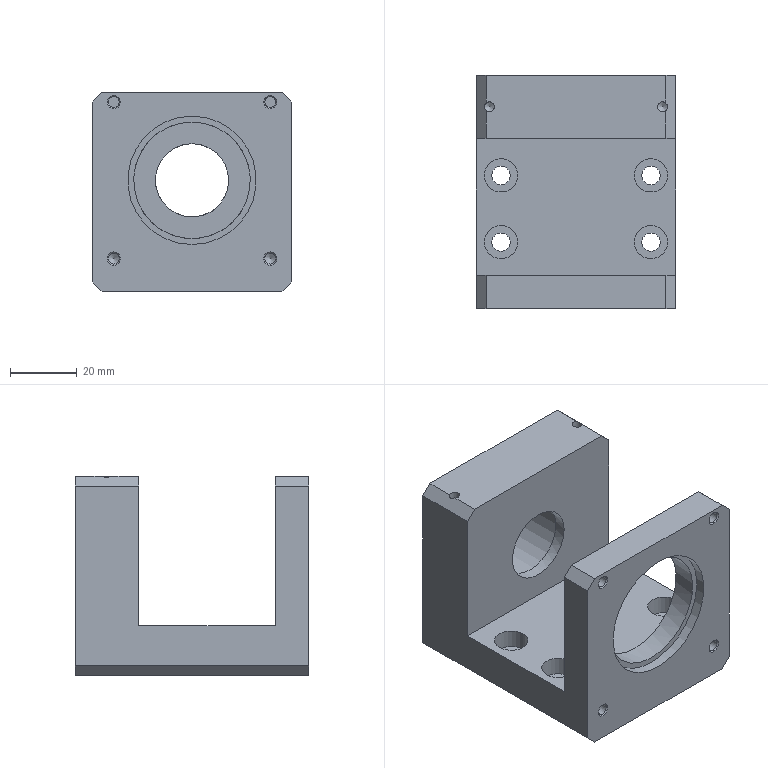Part | NX | 1 solid | 62 faces | box 60 x 70 x 60 mm | volume 117109 mm3 | cylinder 22 | plane 22 | cone 18 | commonest cylinder face diameters 3 x6 3.3 x4 5.5 x4 10 x4 22 x1 26 x1
STEP:
#1=CARTESIAN_POINT('',(41.,-19.,33.5));
#2=VERTEX_POINT('',#1);
#3=CARTESIAN_POINT('',(30.,-19.,33.5));
#4=DIRECTION('',(0.,1.,0.));
#5=DIRECTION('',(1.,0.,0.));
#6=AXIS2_PLACEMENT_3D('',#3,#4,#5);
#7=CIRCLE('',#6,11.);
#8=EDGE_CURVE('',#2,#2,#7,.T.);
#9=ORIENTED_EDGE('',*,*,#8,.F.);
#10=EDGE_LOOP('',(#9));
#11=FACE_BOUND('',#10,.T.);
#12=CARTESIAN_POINT('',(30.,-15.5,44.5));
#13=VERTEX_POINT('',#12);
#14=CARTESIAN_POINT('',(30.,-15.5,33.5));
#15=DIRECTION('',(0.,1.,0.));
#16=DIRECTION('',(0.,0.,1.));
#17=AXIS2_PLACEMENT_3D('',#14,#15,#16);
#18=CIRCLE('',#17,11.);
#19=EDGE_CURVE('',#13,#13,#18,.T.);
#20=ORIENTED_EDGE('',*,*,#19,.T.);
#21=EDGE_LOOP('',(#20));
#22=FACE_BOUND('',#21,.T.);
#23=CARTESIAN_POINT('',(30.,30.,33.5));
#24=DIRECTION('',(0.,-1.,0.));
#25=DIRECTION('',(0.,0.,1.));
#26=AXIS2_PLACEMENT_3D('',#23,#24,#25);
#27=CYLINDRICAL_SURFACE('',#26,11.);
#28=ADVANCED_FACE('',(#11,#22),#27,.F.);
#29=CARTESIAN_POINT('',(55.25,-30.,0.));
#30=VERTEX_POINT('',#29);
#31=CARTESIAN_POINT('',(52.5,-30.,0.));
#32=DIRECTION('',(0.,0.,1.));
#33=DIRECTION('',(1.,0.,0.));
#34=AXIS2_PLACEMENT_3D('',#31,#32,#33);
#35=CIRCLE('',#34,2.75);
#36=EDGE_CURVE('',#30,#30,#35,.T.);
#37=ORIENTED_EDGE('',*,*,#36,.F.);
#38=EDGE_LOOP('',(#37));
#39=FACE_BOUND('',#38,.T.);
#40=CARTESIAN_POINT('',(55.25,-30.,9.3));
#41=VERTEX_POINT('',#40);
#42=CARTESIAN_POINT('',(52.5,-30.,9.3));
#43=DIRECTION('',(0.,0.,-1.));
#44=DIRECTION('',(1.,0.,0.));
#45=AXIS2_PLACEMENT_3D('',#42,#43,#44);
#46=CIRCLE('',#45,2.75);
#47=EDGE_CURVE('',#41,#41,#46,.T.);
#48=ORIENTED_EDGE('',*,*,#47,.F.);
#49=EDGE_LOOP('',(#48));
#50=FACE_BOUND('',#49,.T.);
#51=CARTESIAN_POINT('',(52.5,-30.,-140.));
#52=DIRECTION('',(0.,0.,1.));
#53=DIRECTION('',(-1.,0.,0.));
#54=AXIS2_PLACEMENT_3D('',#51,#52,#53);
#55=CYLINDRICAL_SURFACE('',#54,2.75);
#56=ADVANCED_FACE('',(#39,#50),#55,.F.);
#57=CARTESIAN_POINT('',(10.25,-50.,0.));
#58=VERTEX_POINT('',#57);
#59=CARTESIAN_POINT('',(7.5,-50.,0.));
#60=DIRECTION('',(0.,0.,1.));
#61=DIRECTION('',(1.,0.,0.));
#62=AXIS2_PLACEMENT_3D('',#59,#60,#61);
#63=CIRCLE('',#62,2.75);
#64=EDGE_CURVE('',#58,#58,#63,.T.);
#65=ORIENTED_EDGE('',*,*,#64,.F.);
#66=EDGE_LOOP('',(#65));
#67=FACE_BOUND('',#66,.T.);
#68=CARTESIAN_POINT('',(10.25,-50.,9.3));
#69=VERTEX_POINT('',#68);
#70=CARTESIAN_POINT('',(7.5,-50.,9.3));
#71=DIRECTION('',(0.,0.,-1.));
#72=DIRECTION('',(1.,0.,0.));
#73=AXIS2_PLACEMENT_3D('',#70,#71,#72);
#74=CIRCLE('',#73,2.75);
#75=EDGE_CURVE('',#69,#69,#74,.T.);
#76=ORIENTED_EDGE('',*,*,#75,.F.);
#77=EDGE_LOOP('',(#76));
#78=FACE_BOUND('',#77,.T.);
#79=CARTESIAN_POINT('',(7.5,-50.,-140.));
#80=DIRECTION('',(0.,0.,1.));
#81=DIRECTION('',(-1.,0.,0.));
#82=AXIS2_PLACEMENT_3D('',#79,#80,#81);
#83=CYLINDRICAL_SURFACE('',#82,2.75);
#84=ADVANCED_FACE('',(#67,#78),#83,.F.);
#85=CARTESIAN_POINT('',(10.25,-30.,0.));
#86=VERTEX_POINT('',#85);
#87=CARTESIAN_POINT('',(7.5,-30.,0.));
#88=DIRECTION('',(0.,0.,1.));
#89=DIRECTION('',(1.,0.,0.));
#90=AXIS2_PLACEMENT_3D('',#87,#88,#89);
#91=CIRCLE('',#90,2.75);
#92=EDGE_CURVE('',#86,#86,#91,.T.);
#93=ORIENTED_EDGE('',*,*,#92,.F.);
#94=EDGE_LOOP('',(#93));
#95=FACE_BOUND('',#94,.T.);
#96=CARTESIAN_POINT('',(10.25,-30.,9.3));
#97=VERTEX_POINT('',#96);
#98=CARTESIAN_POINT('',(7.5,-30.,9.3));
#99=DIRECTION('',(0.,0.,-1.));
#100=DIRECTION('',(1.,0.,0.));
#101=AXIS2_PLACEMENT_3D('',#98,#99,#100);
#102=CIRCLE('',#101,2.75);
#103=EDGE_CURVE('',#97,#97,#102,.T.);
#104=ORIENTED_EDGE('',*,*,#103,.F.);
#105=EDGE_LOOP('',(#104));
#106=FACE_BOUND('',#105,.T.);
#107=CARTESIAN_POINT('',(7.5,-30.,-140.));
#108=DIRECTION('',(0.,0.,1.));
#109=DIRECTION('',(-1.,0.,0.));
#110=AXIS2_PLACEMENT_3D('',#107,#108,#109);
#111=CYLINDRICAL_SURFACE('',#110,2.75);
#112=ADVANCED_FACE('',(#95,#106),#111,.F.);
#113=CARTESIAN_POINT('',(55.25,-50.,0.));
#114=VERTEX_POINT('',#113);
#115=CARTESIAN_POINT('',(52.5,-50.,0.));
#116=DIRECTION('',(0.,0.,1.));
#117=DIRECTION('',(1.,0.,0.));
#118=AXIS2_PLACEMENT_3D('',#115,#116,#117);
#119=CIRCLE('',#118,2.75);
#120=EDGE_CURVE('',#114,#114,#119,.T.);
#121=ORIENTED_EDGE('',*,*,#120,.F.);
#122=EDGE_LOOP('',(#121));
#123=FACE_BOUND('',#122,.T.);
#124=CARTESIAN_POINT('',(55.25,-50.,9.3));
#125=VERTEX_POINT('',#124);
#126=CARTESIAN_POINT('',(52.5,-50.,9.3));
#127=DIRECTION('',(0.,0.,-1.));
#128=DIRECTION('',(1.,0.,0.));
#129=AXIS2_PLACEMENT_3D('',#126,#127,#128);
#130=CIRCLE('',#129,2.75);
#131=EDGE_CURVE('',#125,#125,#130,.T.);
#132=ORIENTED_EDGE('',*,*,#131,.F.);
#133=EDGE_LOOP('',(#132));
#134=FACE_BOUND('',#133,.T.);
#135=CARTESIAN_POINT('',(52.5,-50.,-140.));
#136=DIRECTION('',(0.,0.,1.));
#137=DIRECTION('',(-1.,0.,0.));
#138=AXIS2_PLACEMENT_3D('',#135,#136,#137);
#139=CYLINDRICAL_SURFACE('',#138,2.75);
#140=ADVANCED_FACE('',(#123,#134),#139,.F.);
#141=CARTESIAN_POINT('',(57.,-60.,60.));
#142=VERTEX_POINT('',#141);
#143=CARTESIAN_POINT('',(57.,-70.,60.));
#144=VERTEX_POINT('',#143);
#145=CARTESIAN_POINT('',(57.,0.,60.));
#146=DIRECTION('',(0.,-1.,0.));
#147=VECTOR('',#146,1.);
#148=LINE('',#145,#147);
#149=EDGE_CURVE('',#142,#144,#148,.T.);
#150=ORIENTED_EDGE('',*,*,#149,.F.);
#151=CARTESIAN_POINT('',(3.,-60.,60.));
#152=VERTEX_POINT('',#151);
#153=CARTESIAN_POINT('',(60.,-60.,60.));
#154=DIRECTION('',(-1.,0.,0.));
#155=VECTOR('',#154,1.);
#156=LINE('',#153,#155);
#157=EDGE_CURVE('',#142,#152,#156,.T.);
#158=ORIENTED_EDGE('',*,*,#157,.T.);
#159=CARTESIAN_POINT('',(3.,-70.,60.));
#160=VERTEX_POINT('',#159);
#161=CARTESIAN_POINT('',(3.,0.,60.));
#162=DIRECTION('',(0.,-1.,0.));
#163=VECTOR('',#162,1.);
#164=LINE('',#161,#163);
#165=EDGE_CURVE('',#152,#160,#164,.T.);
#166=ORIENTED_EDGE('',*,*,#165,.T.);
#167=CARTESIAN_POINT('',(3.,-70.,60.));
#168=DIRECTION('',(1.,0.,0.));
#169=VECTOR('',#168,1.);
#170=LINE('',#167,#169);
#171=EDGE_CURVE('',#160,#144,#170,.T.);
#172=ORIENTED_EDGE('',*,*,#171,.T.);
#173=EDGE_LOOP('',(#150,#158,#166,#172));
#174=FACE_OUTER_BOUND('',#173,.T.);
#175=CARTESIAN_POINT('',(3.,0.,60.));
#176=DIRECTION('',(0.,0.,-1.));
#177=DIRECTION('',(1.,0.,0.));
#178=AXIS2_PLACEMENT_3D('',#175,#176,#177);
#179=PLANE('',#178);
#180=ADVANCED_FACE('',(#174),#179,.F.);
#181=CARTESIAN_POINT('',(57.,0.,60.));
#182=VERTEX_POINT('',#181);
#183=CARTESIAN_POINT('',(57.,-8.382,60.));
#184=VERTEX_POINT('',#183);
#185=CARTESIAN_POINT('',(57.,0.,60.));
#186=DIRECTION('',(0.,-1.,0.));
#187=VECTOR('',#186,1.);
#188=LINE('',#185,#187);
#189=EDGE_CURVE('',#182,#184,#188,.T.);
#190=ORIENTED_EDGE('',*,*,#189,.T.);
#191=CARTESIAN_POINT('',(57.,-10.618,60.));
#192=VERTEX_POINT('',#191);
#193=CARTESIAN_POINT('',(56.,-9.5,61.));
#194=DIRECTION('',(-0.7071,0.,-0.7071));
#195=DIRECTION('',(0.7071,0.,-0.7071));
#196=AXIS2_PLACEMENT_3D('',#193,#194,#195);
#197=ELLIPSE('',#196,2.121,1.5);
#198=EDGE_CURVE('',#184,#192,#197,.T.);
#199=ORIENTED_EDGE('',*,*,#198,.T.);
#200=CARTESIAN_POINT('',(57.,-19.,60.));
#201=VERTEX_POINT('',#200);
#202=CARTESIAN_POINT('',(57.,0.,60.));
#203=DIRECTION('',(0.,-1.,0.));
#204=VECTOR('',#203,1.);
#205=LINE('',#202,#204);
#206=EDGE_CURVE('',#192,#201,#205,.T.);
#207=ORIENTED_EDGE('',*,*,#206,.T.);
#208=CARTESIAN_POINT('',(60.,-19.,57.));
#209=VERTEX_POINT('',#208);
#210=CARTESIAN_POINT('',(57.,-19.,60.));
#211=DIRECTION('',(-0.7071,0.,0.7071));
#212=VECTOR('',#211,1.);
#213=LINE('',#210,#212);
#214=EDGE_CURVE('',#209,#201,#213,.T.);
#215=ORIENTED_EDGE('',*,*,#214,.F.);
#216=CARTESIAN_POINT('',(60.,0.,57.));
#217=VERTEX_POINT('',#216);
#218=CARTESIAN_POINT('',(60.,0.,57.));
#219=DIRECTION('',(0.,-1.,0.));
#220=VECTOR('',#219,1.);
#221=LINE('',#218,#220);
#222=EDGE_CURVE('',#217,#209,#221,.T.);
#223=ORIENTED_EDGE('',*,*,#222,.F.);
#224=CARTESIAN_POINT('',(57.,0.,60.));
#225=DIRECTION('',(0.7071,0.,-0.7071));
#226=VECTOR('',#225,1.);
#227=LINE('',#224,#226);
#228=EDGE_CURVE('',#182,#217,#227,.T.);
#229=ORIENTED_EDGE('',*,*,#228,.F.);
#230=EDGE_LOOP('',(#190,#199,#207,#215,#223,#229));
#231=FACE_OUTER_BOUND('',#230,.T.);
#232=CARTESIAN_POINT('',(57.,0.,60.));
#233=DIRECTION('',(-0.7071,0.,-0.7071));
#234=DIRECTION('',(0.7071,0.,-0.7071));
#235=AXIS2_PLACEMENT_3D('',#232,#233,#234);
#236=PLANE('',#235);
#237=ADVANCED_FACE('',(#231),#236,.F.);
#238=CARTESIAN_POINT('',(60.,-60.,57.));
#239=VERTEX_POINT('',#238);
#240=CARTESIAN_POINT('',(57.,-60.,60.));
#241=DIRECTION('',(0.7071,0.,-0.7071));
#242=VECTOR('',#241,1.);
#243=LINE('',#240,#242);
#244=EDGE_CURVE('',#142,#239,#243,.T.);
#245=ORIENTED_EDGE('',*,*,#244,.F.);
#246=ORIENTED_EDGE('',*,*,#149,.T.);
#247=CARTESIAN_POINT('',(60.,-70.,57.));
#248=VERTEX_POINT('',#247);
#249=CARTESIAN_POINT('',(57.,-70.,60.));
#250=DIRECTION('',(0.7071,0.,-0.7071));
#251=VECTOR('',#250,1.);
#252=LINE('',#249,#251);
#253=EDGE_CURVE('',#144,#248,#252,.T.);
#254=ORIENTED_EDGE('',*,*,#253,.T.);
#255=CARTESIAN_POINT('',(60.,0.,57.));
#256=DIRECTION('',(0.,-1.,0.));
#257=VECTOR('',#256,1.);
#258=LINE('',#255,#257);
#259=EDGE_CURVE('',#239,#248,#258,.T.);
#260=ORIENTED_EDGE('',*,*,#259,.F.);
#261=EDGE_LOOP('',(#245,#246,#254,#260));
#262=FACE_OUTER_BOUND('',#261,.T.);
#263=CARTESIAN_POINT('',(57.,0.,60.));
#264=DIRECTION('',(-0.7071,0.,-0.7071));
#265=DIRECTION('',(0.7071,0.,-0.7071));
#266=AXIS2_PLACEMENT_3D('',#263,#264,#265);
#267=PLANE('',#266);
#268=ADVANCED_FACE('',(#262),#267,.F.);
#269=CARTESIAN_POINT('',(3.,-10.618,60.));
#270=VERTEX_POINT('',#269);
#271=CARTESIAN_POINT('',(3.,-19.,60.));
#272=VERTEX_POINT('',#271);
#273=CARTESIAN_POINT('',(3.,0.,60.));
#274=DIRECTION('',(0.,-1.,0.));
#275=VECTOR('',#274,1.);
#276=LINE('',#273,#275);
#277=EDGE_CURVE('',#270,#272,#276,.T.);
#278=ORIENTED_EDGE('',*,*,#277,.F.);
#279=CARTESIAN_POINT('',(3.,-8.382,60.));
#280=VERTEX_POINT('',#279);
#281=CARTESIAN_POINT('',(4.,-9.5,61.));
#282=DIRECTION('',(0.7071,0.,-0.7071));
#283=DIRECTION('',(-0.7071,0.,-0.7071));
#284=AXIS2_PLACEMENT_3D('',#281,#282,#283);
#285=ELLIPSE('',#284,2.121,1.5);
#286=EDGE_CURVE('',#270,#280,#285,.T.);
#287=ORIENTED_EDGE('',*,*,#286,.T.);
#288=CARTESIAN_POINT('',(3.,0.,60.));
#289=VERTEX_POINT('',#288);
#290=CARTESIAN_POINT('',(3.,0.,60.));
#291=DIRECTION('',(0.,-1.,0.));
#292=VECTOR('',#291,1.);
#293=LINE('',#290,#292);
#294=EDGE_CURVE('',#289,#280,#293,.T.);
#295=ORIENTED_EDGE('',*,*,#294,.F.);
#296=CARTESIAN_POINT('',(0.,0.,57.));
#297=VERTEX_POINT('',#296);
#298=CARTESIAN_POINT('',(0.,0.,57.));
#299=DIRECTION('',(0.7071,0.,0.7071));
#300=VECTOR('',#299,1.);
#301=LINE('',#298,#300);
#302=EDGE_CURVE('',#297,#289,#301,.T.);
#303=ORIENTED_EDGE('',*,*,#302,.F.);
#304=CARTESIAN_POINT('',(0.,-19.,57.));
#305=VERTEX_POINT('',#304);
#306=CARTESIAN_POINT('',(0.,0.,57.));
#307=DIRECTION('',(0.,-1.,0.));
#308=VECTOR('',#307,1.);
#309=LINE('',#306,#308);
#310=EDGE_CURVE('',#297,#305,#309,.T.);
#311=ORIENTED_EDGE('',*,*,#310,.T.);
#312=CARTESIAN_POINT('',(0.,-19.,57.));
#313=DIRECTION('',(-0.7071,0.,-0.7071));
#314=VECTOR('',#313,1.);
#315=LINE('',#312,#314);
#316=EDGE_CURVE('',#272,#305,#315,.T.);
#317=ORIENTED_EDGE('',*,*,#316,.F.);
#318=EDGE_LOOP('',(#278,#287,#295,#303,#311,#317));
#319=FACE_OUTER_BOUND('',#318,.T.);
#320=CARTESIAN_POINT('',(0.,0.,57.));
#321=DIRECTION('',(0.7071,0.,-0.7071));
#322=DIRECTION('',(0.7071,0.,0.7071));
#323=AXIS2_PLACEMENT_3D('',#320,#321,#322);
#324=PLANE('',#323);
#325=ADVANCED_FACE('',(#319),#324,.F.);
#326=CARTESIAN_POINT('',(0.,-60.,57.));
#327=VERTEX_POINT('',#326);
#328=CARTESIAN_POINT('',(0.,-60.,57.));
#329=DIRECTION('',(0.7071,0.,0.7071));
#330=VECTOR('',#329,1.);
#331=LINE('',#328,#330);
#332=EDGE_CURVE('',#327,#152,#331,.T.);
#333=ORIENTED_EDGE('',*,*,#332,.F.);
#334=CARTESIAN_POINT('',(0.,-70.,57.));
#335=VERTEX_POINT('',#334);
#336=CARTESIAN_POINT('',(0.,0.,57.));
#337=DIRECTION('',(0.,-1.,0.));
#338=VECTOR('',#337,1.);
#339=LINE('',#336,#338);
#340=EDGE_CURVE('',#327,#335,#339,.T.);
#341=ORIENTED_EDGE('',*,*,#340,.T.);
#342=CARTESIAN_POINT('',(0.,-70.,57.));
#343=DIRECTION('',(0.7071,0.,0.7071));
#344=VECTOR('',#343,1.);
#345=LINE('',#342,#344);
#346=EDGE_CURVE('',#335,#160,#345,.T.);
#347=ORIENTED_EDGE('',*,*,#346,.T.);
#348=ORIENTED_EDGE('',*,*,#165,.F.);
#349=EDGE_LOOP('',(#333,#341,#347,#348));
#350=FACE_OUTER_BOUND('',#349,.T.);
#351=CARTESIAN_POINT('',(0.,0.,57.));
#352=DIRECTION('',(0.7071,0.,-0.7071));
#353=DIRECTION('',(0.7071,0.,0.7071));
#354=AXIS2_PLACEMENT_3D('',#351,#352,#353);
#355=PLANE('',#354);
#356=ADVANCED_FACE('',(#350),#355,.F.);
#357=ORIENTED_EDGE('',*,*,#206,.F.);
#358=CARTESIAN_POINT('',(56.,-9.5,60.));
#359=DIRECTION('',(0.,0.,-1.));
#360=DIRECTION('',(-1.,0.,0.));
#361=AXIS2_PLACEMENT_3D('',#358,#359,#360);
#362=CIRCLE('',#361,1.5);
#363=EDGE_CURVE('',#192,#184,#362,.T.);
#364=ORIENTED_EDGE('',*,*,#363,.T.);
#365=ORIENTED_EDGE('',*,*,#189,.F.);
#366=CARTESIAN_POINT('',(3.,0.,60.));
#367=DIRECTION('',(1.,0.,0.));
#368=VECTOR('',#367,1.);
#369=LINE('',#366,#368);
#370=EDGE_CURVE('',#289,#182,#369,.T.);
#371=ORIENTED_EDGE('',*,*,#370,.F.);
#372=ORIENTED_EDGE('',*,*,#294,.T.);
#373=CARTESIAN_POINT('',(4.,-9.5,60.));
#374=DIRECTION('',(0.,0.,-1.));
#375=DIRECTION('',(-1.,0.,0.));
#376=AXIS2_PLACEMENT_3D('',#373,#374,#375);
#377=CIRCLE('',#376,1.5);
#378=EDGE_CURVE('',#280,#270,#377,.T.);
#379=ORIENTED_EDGE('',*,*,#378,.T.);
#380=ORIENTED_EDGE('',*,*,#277,.T.);
#381=CARTESIAN_POINT('',(0.,-19.,60.));
#382=DIRECTION('',(1.,0.,0.));
#383=VECTOR('',#382,1.);
#384=LINE('',#381,#383);
#385=EDGE_CURVE('',#272,#201,#384,.T.);
#386=ORIENTED_EDGE('',*,*,#385,.T.);
#387=EDGE_LOOP('',(#357,#364,#365,#371,#372,#379,#380,#386));
#388=FACE_OUTER_BOUND('',#387,.T.);
#389=CARTESIAN_POINT('',(3.,0.,60.));
#390=DIRECTION('',(0.,0.,-1.));
#391=DIRECTION('',(1.,0.,0.));
#392=AXIS2_PLACEMENT_3D('',#389,#390,#391);
#393=PLANE('',#392);
#394=ADVANCED_FACE('',(#388),#393,.F.);
#395=CARTESIAN_POINT('',(60.,-19.,15.));
#396=VERTEX_POINT('',#395);
#397=CARTESIAN_POINT('',(60.,-60.,15.));
#398=VERTEX_POINT('',#397);
#399=CARTESIAN_POINT('',(60.,-19.,15.));
#400=DIRECTION('',(0.,-1.,0.));
#401=VECTOR('',#400,1.);
#402=LINE('',#399,#401);
#403=EDGE_CURVE('',#396,#398,#402,.T.);
#404=ORIENTED_EDGE('',*,*,#403,.T.);
#405=CARTESIAN_POINT('',(60.,-60.,15.));
#406=DIRECTION('',(0.,0.,1.));
#407=VECTOR('',#406,1.);
#408=LINE('',#405,#407);
#409=EDGE_CURVE('',#398,#239,#408,.T.);
#410=ORIENTED_EDGE('',*,*,#409,.T.);
#411=ORIENTED_EDGE('',*,*,#259,.T.);
#412=CARTESIAN_POINT('',(60.,-70.,3.));
#413=VERTEX_POINT('',#412);
#414=CARTESIAN_POINT('',(60.,-70.,57.));
#415=DIRECTION('',(0.,0.,-1.));
#416=VECTOR('',#415,1.);
#417=LINE('',#414,#416);
#418=EDGE_CURVE('',#248,#413,#417,.T.);
#419=ORIENTED_EDGE('',*,*,#418,.T.);
#420=CARTESIAN_POINT('',(60.,0.,3.));
#421=VERTEX_POINT('',#420);
#422=CARTESIAN_POINT('',(60.,0.,3.));
#423=DIRECTION('',(0.,-1.,0.));
#424=VECTOR('',#423,1.);
#425=LINE('',#422,#424);
#426=EDGE_CURVE('',#421,#413,#425,.T.);
#427=ORIENTED_EDGE('',*,*,#426,.F.);
#428=CARTESIAN_POINT('',(60.,0.,57.));
#429=DIRECTION('',(0.,0.,-1.));
#430=VECTOR('',#429,1.);
#431=LINE('',#428,#430);
#432=EDGE_CURVE('',#217,#421,#431,.T.);
#433=ORIENTED_EDGE('',*,*,#432,.F.);
#434=ORIENTED_EDGE('',*,*,#222,.T.);
#435=CARTESIAN_POINT('',(60.,-19.,15.));
#436=DIRECTION('',(0.,0.,1.));
#437=VECTOR('',#436,1.);
#438=LINE('',#435,#437);
#439=EDGE_CURVE('',#396,#209,#438,.T.);
#440=ORIENTED_EDGE('',*,*,#439,.F.);
#441=EDGE_LOOP('',(#404,#410,#411,#419,#427,#433,#434,#440));
#442=FACE_OUTER_BOUND('',#441,.T.);
#443=CARTESIAN_POINT('',(60.,0.,57.));
#444=DIRECTION('',(-1.,0.,0.));
#445=DIRECTION('',(0.,0.,-1.));
#446=AXIS2_PLACEMENT_3D('',#443,#444,#445);
#447=PLANE('',#446);
#448=ADVANCED_FACE('',(#442),#447,.F.);
#449=CARTESIAN_POINT('',(57.,-70.,0.));
#450=VERTEX_POINT('',#449);
#451=CARTESIAN_POINT('',(60.,-70.,3.));
#452=DIRECTION('',(-0.7071,0.,-0.7071));
#453=VECTOR('',#452,1.);
#454=LINE('',#451,#453);
#455=EDGE_CURVE('',#413,#450,#454,.T.);
#456=ORIENTED_EDGE('',*,*,#455,.T.);
#457=CARTESIAN_POINT('',(57.,0.,0.));
#458=VERTEX_POINT('',#457);
#459=CARTESIAN_POINT('',(57.,0.,0.));
#460=DIRECTION('',(0.,-1.,0.));
#461=VECTOR('',#460,1.);
#462=LINE('',#459,#461);
#463=EDGE_CURVE('',#458,#450,#462,.T.);
#464=ORIENTED_EDGE('',*,*,#463,.F.);
#465=CARTESIAN_POINT('',(60.,0.,3.));
#466=DIRECTION('',(-0.7071,0.,-0.7071));
#467=VECTOR('',#466,1.);
#468=LINE('',#465,#467);
#469=EDGE_CURVE('',#421,#458,#468,.T.);
#470=ORIENTED_EDGE('',*,*,#469,.F.);
#471=ORIENTED_EDGE('',*,*,#426,.T.);
#472=EDGE_LOOP('',(#456,#464,#470,#471));
#473=FACE_OUTER_BOUND('',#472,.T.);
#474=CARTESIAN_POINT('',(60.,0.,3.));
#475=DIRECTION('',(-0.7071,0.,0.7071));
#476=DIRECTION('',(-0.7071,0.,-0.7071));
#477=AXIS2_PLACEMENT_3D('',#474,#475,#476);
#478=PLANE('',#477);
#479=ADVANCED_FACE('',(#473),#478,.F.);
#480=ORIENTED_EDGE('',*,*,#120,.T.);
#481=EDGE_LOOP('',(#480));
#482=FACE_BOUND('',#481,.T.);
#483=ORIENTED_EDGE('',*,*,#92,.T.);
#484=EDGE_LOOP('',(#483));
#485=FACE_BOUND('',#484,.T.);
#486=ORIENTED_EDGE('',*,*,#64,.T.);
#487=EDGE_LOOP('',(#486));
#488=FACE_BOUND('',#487,.T.);
#489=ORIENTED_EDGE('',*,*,#36,.T.);
#490=EDGE_LOOP('',(#489));
#491=FACE_BOUND('',#490,.T.);
#492=CARTESIAN_POINT('',(3.,-70.,0.));
#493=VERTEX_POINT('',#492);
#494=CARTESIAN_POINT('',(57.,-70.,0.));
#495=DIRECTION('',(-1.,0.,0.));
#496=VECTOR('',#495,1.);
#497=LINE('',#494,#496);
#498=EDGE_CURVE('',#450,#493,#497,.T.);
#499=ORIENTED_EDGE('',*,*,#498,.T.);
#500=CARTESIAN_POINT('',(3.,0.,0.));
#501=VERTEX_POINT('',#500);
#502=CARTESIAN_POINT('',(3.,0.,0.));
#503=DIRECTION('',(0.,-1.,0.));
#504=VECTOR('',#503,1.);
#505=LINE('',#502,#504);
#506=EDGE_CURVE('',#501,#493,#505,.T.);
#507=ORIENTED_EDGE('',*,*,#506,.F.);
#508=CARTESIAN_POINT('',(57.,0.,0.));
#509=DIRECTION('',(-1.,0.,0.));
#510=VECTOR('',#509,1.);
#511=LINE('',#508,#510);
#512=EDGE_CURVE('',#458,#501,#511,.T.);
#513=ORIENTED_EDGE('',*,*,#512,.F.);
#514=ORIENTED_EDGE('',*,*,#463,.T.);
#515=EDGE_LOOP('',(#499,#507,#513,#514));
#516=FACE_BOUND('',#515,.T.);
#517=CARTESIAN_POINT('',(57.,0.,0.));
#518=DIRECTION('',(0.,0.,1.));
#519=DIRECTION('',(-1.,0.,0.));
#520=AXIS2_PLACEMENT_3D('',#517,#518,#519);
#521=PLANE('',#520);
#522=ADVANCED_FACE('',(#482,#485,#488,#491,#516),#521,.F.);
#523=CARTESIAN_POINT('',(0.,-70.,3.));
#524=VERTEX_POINT('',#523);
#525=CARTESIAN_POINT('',(3.,-70.,0.));
#526=DIRECTION('',(-0.7071,0.,0.7071));
#527=VECTOR('',#526,1.);
#528=LINE('',#525,#527);
#529=EDGE_CURVE('',#493,#524,#528,.T.);
#530=ORIENTED_EDGE('',*,*,#529,.T.);
#531=CARTESIAN_POINT('',(0.,0.,3.));
#532=VERTEX_POINT('',#531);
#533=CARTESIAN_POINT('',(0.,0.,3.));
#534=DIRECTION('',(0.,-1.,0.));
#535=VECTOR('',#534,1.);
#536=LINE('',#533,#535);
#537=EDGE_CURVE('',#532,#524,#536,.T.);
#538=ORIENTED_EDGE('',*,*,#537,.F.);
#539=CARTESIAN_POINT('',(3.,0.,0.));
#540=DIRECTION('',(-0.7071,0.,0.7071));
#541=VECTOR('',#540,1.);
#542=LINE('',#539,#541);
#543=EDGE_CURVE('',#501,#532,#542,.T.);
#544=ORIENTED_EDGE('',*,*,#543,.F.);
#545=ORIENTED_EDGE('',*,*,#506,.T.);
#546=EDGE_LOOP('',(#530,#538,#544,#545));
#547=FACE_OUTER_BOUND('',#546,.T.);
#548=CARTESIAN_POINT('',(3.,0.,0.));
#549=DIRECTION('',(0.7071,0.,0.7071));
#550=DIRECTION('',(-0.7071,0.,0.7071));
#551=AXIS2_PLACEMENT_3D('',#548,#549,#550);
#552=PLANE('',#551);
#553=ADVANCED_FACE('',(#547),#552,.F.);
#554=CARTESIAN_POINT('',(0.,-60.,15.));
#555=VERTEX_POINT('',#554);
#556=CARTESIAN_POINT('',(0.,-19.,15.));
#557=VERTEX_POINT('',#556);
#558=CARTESIAN_POINT('',(0.,-60.,15.));
#559=DIRECTION('',(0.,1.,0.));
#560=VECTOR('',#559,1.);
#561=LINE('',#558,#560);
#562=EDGE_CURVE('',#555,#557,#561,.T.);
#563=ORIENTED_EDGE('',*,*,#562,.T.);
#564=CARTESIAN_POINT('',(0.,-19.,15.));
#565=DIRECTION('',(0.,0.,1.));
#566=VECTOR('',#565,1.);
#567=LINE('',#564,#566);
#568=EDGE_CURVE('',#557,#305,#567,.T.);
#569=ORIENTED_EDGE('',*,*,#568,.T.);
#570=ORIENTED_EDGE('',*,*,#310,.F.);
#571=CARTESIAN_POINT('',(0.,0.,3.));
#572=DIRECTION('',(0.,0.,1.));
#573=VECTOR('',#572,1.);
#574=LINE('',#571,#573);
#575=EDGE_CURVE('',#532,#297,#574,.T.);
#576=ORIENTED_EDGE('',*,*,#575,.F.);
#577=ORIENTED_EDGE('',*,*,#537,.T.);
#578=CARTESIAN_POINT('',(0.,-70.,3.));
#579=DIRECTION('',(0.,0.,1.));
#580=VECTOR('',#579,1.);
#581=LINE('',#578,#580);
#582=EDGE_CURVE('',#524,#335,#581,.T.);
#583=ORIENTED_EDGE('',*,*,#582,.T.);
#584=ORIENTED_EDGE('',*,*,#340,.F.);
#585=CARTESIAN_POINT('',(0.,-60.,15.));
#586=DIRECTION('',(0.,0.,1.));
#587=VECTOR('',#586,1.);
#588=LINE('',#585,#587);
#589=EDGE_CURVE('',#555,#327,#588,.T.);
#590=ORIENTED_EDGE('',*,*,#589,.F.);
#591=EDGE_LOOP('',(#563,#569,#570,#576,#577,#583,#584,#590));
#592=FACE_OUTER_BOUND('',#591,.T.);
#593=CARTESIAN_POINT('',(0.,0.,3.));
#594=DIRECTION('',(1.,0.,0.));
#595=DIRECTION('',(0.,0.,1.));
#596=AXIS2_PLACEMENT_3D('',#593,#594,#595);
#597=PLANE('',#596);
#598=ADVANCED_FACE('',(#592),#597,.F.);
#599=CARTESIAN_POINT('',(42.5,0.,22.75));
#600=VERTEX_POINT('',#599);
#601=CARTESIAN_POINT('',(42.5,0.,21.));
#602=DIRECTION('',(0.,-1.,0.));
#603=DIRECTION('',(0.,0.,1.));
#604=AXIS2_PLACEMENT_3D('',#601,#602,#603);
#605=CIRCLE('',#604,1.75);
#606=EDGE_CURVE('',#600,#600,#605,.T.);
#607=ORIENTED_EDGE('',*,*,#606,.T.);
#608=EDGE_LOOP('',(#607));
#609=FACE_BOUND('',#608,.T.);
#610=CARTESIAN_POINT('',(17.5,0.,22.75));
#611=VERTEX_POINT('',#610);
#612=CARTESIAN_POINT('',(17.5,0.,21.));
#613=DIRECTION('',(0.,-1.,0.));
#614=DIRECTION('',(0.,0.,1.));
#615=AXIS2_PLACEMENT_3D('',#612,#613,#614);
#616=CIRCLE('',#615,1.75);
#617=EDGE_CURVE('',#611,#611,#616,.T.);
#618=ORIENTED_EDGE('',*,*,#617,.T.);
#619=EDGE_LOOP('',(#618));
#620=FACE_BOUND('',#619,.T.);
#621=CARTESIAN_POINT('',(17.5,0.,47.75));
#622=VERTEX_POINT('',#621);
#623=CARTESIAN_POINT('',(17.5,0.,46.));
#624=DIRECTION('',(0.,-1.,0.));
#625=DIRECTION('',(0.,0.,1.));
#626=AXIS2_PLACEMENT_3D('',#623,#624,#625);
#627=CIRCLE('',#626,1.75);
#628=EDGE_CURVE('',#622,#622,#627,.T.);
#629=ORIENTED_EDGE('',*,*,#628,.T.);
#630=EDGE_LOOP('',(#629));
#631=FACE_BOUND('',#630,.T.);
#632=CARTESIAN_POINT('',(42.5,0.,47.75));
#633=VERTEX_POINT('',#632);
#634=CARTESIAN_POINT('',(42.5,0.,46.));
#635=DIRECTION('',(0.,-1.,0.));
#636=DIRECTION('',(0.,0.,1.));
#637=AXIS2_PLACEMENT_3D('',#634,#635,#636);
#638=CIRCLE('',#637,1.75);
#639=EDGE_CURVE('',#633,#633,#638,.T.);
#640=ORIENTED_EDGE('',*,*,#639,.T.);
#641=EDGE_LOOP('',(#640));
#642=FACE_BOUND('',#641,.T.);
#643=CARTESIAN_POINT('',(30.,0.,46.5));
#644=VERTEX_POINT('',#643);
#645=CARTESIAN_POINT('',(30.,0.,33.5));
#646=DIRECTION('',(0.,-1.,0.));
#647=DIRECTION('',(0.,0.,1.));
#648=AXIS2_PLACEMENT_3D('',#645,#646,#647);
#649=CIRCLE('',#648,13.);
#650=EDGE_CURVE('',#644,#644,#649,.T.);
#651=ORIENTED_EDGE('',*,*,#650,.T.);
#652=EDGE_LOOP('',(#651));
#653=FACE_BOUND('',#652,.T.);
#654=ORIENTED_EDGE('',*,*,#370,.T.);
#655=ORIENTED_EDGE('',*,*,#228,.T.);
#656=ORIENTED_EDGE('',*,*,#432,.T.);
#657=ORIENTED_EDGE('',*,*,#469,.T.);
#658=ORIENTED_EDGE('',*,*,#512,.T.);
#659=ORIENTED_EDGE('',*,*,#543,.T.);
#660=ORIENTED_EDGE('',*,*,#575,.T.);
#661=ORIENTED_EDGE('',*,*,#302,.T.);
#662=EDGE_LOOP('',(#654,#655,#656,#657,#658,#659,#660,#661));
#663=FACE_BOUND('',#662,.T.);
#664=CARTESIAN_POINT('',(0.,0.,0.));
#665=DIRECTION('',(0.,1.,0.));
#666=DIRECTION('',(0.,0.,-1.));
#667=AXIS2_PLACEMENT_3D('',#664,#665,#666);
#668=PLANE('',#667);
#669=ADVANCED_FACE('',(#609,#620,#631,#642,#653,#663),#668,.T.);
#670=CARTESIAN_POINT('',(53.5,-70.,12.));
#671=VERTEX_POINT('',#670);
#672=CARTESIAN_POINT('',(53.5,-70.,10.));
#673=DIRECTION('',(0.,1.,0.));
#674=DIRECTION('',(0.,0.,1.));
#675=AXIS2_PLACEMENT_3D('',#672,#673,#674);
#676=CIRCLE('',#675,2.);
#677=EDGE_CURVE('',#671,#671,#676,.T.);
#678=ORIENTED_EDGE('',*,*,#677,.T.);
#679=EDGE_LOOP('',(#678));
#680=FACE_BOUND('',#679,.T.);
#681=CARTESIAN_POINT('',(6.5,-70.,12.));
#682=VERTEX_POINT('',#681);
#683=CARTESIAN_POINT('',(6.5,-70.,10.));
#684=DIRECTION('',(0.,1.,0.));
#685=DIRECTION('',(0.,0.,1.));
#686=AXIS2_PLACEMENT_3D('',#683,#684,#685);
#687=CIRCLE('',#686,2.);
#688=EDGE_CURVE('',#682,#682,#687,.T.);
#689=ORIENTED_EDGE('',*,*,#688,.T.);
#690=EDGE_LOOP('',(#689));
#691=FACE_BOUND('',#690,.T.);
#692=CARTESIAN_POINT('',(53.5,-70.,59.));
#693=VERTEX_POINT('',#692);
#694=CARTESIAN_POINT('',(53.5,-70.,57.));
#695=DIRECTION('',(0.,1.,0.));
#696=DIRECTION('',(0.,0.,1.));
#697=AXIS2_PLACEMENT_3D('',#694,#695,#696);
#698=CIRCLE('',#697,2.);
#699=EDGE_CURVE('',#693,#693,#698,.T.);
#700=ORIENTED_EDGE('',*,*,#699,.T.);
#701=EDGE_LOOP('',(#700));
#702=FACE_BOUND('',#701,.T.);
#703=CARTESIAN_POINT('',(6.5,-70.,59.));
#704=VERTEX_POINT('',#703);
#705=CARTESIAN_POINT('',(6.5,-70.,57.));
#706=DIRECTION('',(0.,1.,0.));
#707=DIRECTION('',(0.,0.,1.));
#708=AXIS2_PLACEMENT_3D('',#705,#706,#707);
#709=CIRCLE('',#708,2.);
#710=EDGE_CURVE('',#704,#704,#709,.T.);
#711=ORIENTED_EDGE('',*,*,#710,.T.);
#712=EDGE_LOOP('',(#711));
#713=FACE_BOUND('',#712,.T.);
#714=CARTESIAN_POINT('',(30.,-70.,14.25));
#715=VERTEX_POINT('',#714);
#716=CARTESIAN_POINT('',(30.,-70.,33.5));
#717=DIRECTION('',(0.,1.,0.));
#718=DIRECTION('',(0.,0.,-1.));
#719=AXIS2_PLACEMENT_3D('',#716,#717,#718);
#720=CIRCLE('',#719,19.25);
#721=EDGE_CURVE('',#715,#715,#720,.T.);
#722=ORIENTED_EDGE('',*,*,#721,.T.);
#723=EDGE_LOOP('',(#722));
#724=FACE_BOUND('',#723,.T.);
#725=ORIENTED_EDGE('',*,*,#171,.F.);
#726=ORIENTED_EDGE('',*,*,#346,.F.);
#727=ORIENTED_EDGE('',*,*,#582,.F.);
#728=ORIENTED_EDGE('',*,*,#529,.F.);
#729=ORIENTED_EDGE('',*,*,#498,.F.);
#730=ORIENTED_EDGE('',*,*,#455,.F.);
#731=ORIENTED_EDGE('',*,*,#418,.F.);
#732=ORIENTED_EDGE('',*,*,#253,.F.);
#733=EDGE_LOOP('',(#725,#726,#727,#728,#729,#730,#731,#732));
#734=FACE_BOUND('',#733,.T.);
#735=CARTESIAN_POINT('',(0.,-70.,0.));
#736=DIRECTION('',(0.,1.,0.));
#737=DIRECTION('',(0.,0.,-1.));
#738=AXIS2_PLACEMENT_3D('',#735,#736,#737);
#739=PLANE('',#738);
#740=ADVANCED_FACE('',(#680,#691,#702,#713,#724,#734),#739,.F.);
#741=ORIENTED_EDGE('',*,*,#8,.T.);
#742=EDGE_LOOP('',(#741));
#743=FACE_BOUND('',#742,.T.);
#744=ORIENTED_EDGE('',*,*,#214,.T.);
#745=ORIENTED_EDGE('',*,*,#385,.F.);
#746=ORIENTED_EDGE('',*,*,#316,.T.);
#747=ORIENTED_EDGE('',*,*,#568,.F.);
#748=CARTESIAN_POINT('',(0.,-19.,15.));
#749=DIRECTION('',(-1.,0.,0.));
#750=VECTOR('',#749,1.);
#751=LINE('',#748,#750);
#752=EDGE_CURVE('',#396,#557,#751,.T.);
#753=ORIENTED_EDGE('',*,*,#752,.F.);
#754=ORIENTED_EDGE('',*,*,#439,.T.);
#755=EDGE_LOOP('',(#744,#745,#746,#747,#753,#754));
#756=FACE_BOUND('',#755,.T.);
#757=CARTESIAN_POINT('',(0.,-19.,15.));
#758=DIRECTION('',(0.,-1.,0.));
#759=DIRECTION('',(-1.,0.,0.));
#760=AXIS2_PLACEMENT_3D('',#757,#758,#759);
#761=PLANE('',#760);
#762=ADVANCED_FACE('',(#743,#756),#761,.T.);
#763=CARTESIAN_POINT('',(51.5,-60.,57.));
#764=VERTEX_POINT('',#763);
#765=CARTESIAN_POINT('',(53.5,-60.,57.));
#766=DIRECTION('',(0.,-1.,0.));
#767=DIRECTION('',(-1.,0.,0.));
#768=AXIS2_PLACEMENT_3D('',#765,#766,#767);
#769=CIRCLE('',#768,2.);
#770=EDGE_CURVE('',#764,#764,#769,.T.);
#771=ORIENTED_EDGE('',*,*,#770,.T.);
#772=EDGE_LOOP('',(#771));
#773=FACE_BOUND('',#772,.T.);
#774=CARTESIAN_POINT('',(4.5,-60.,57.));
#775=VERTEX_POINT('',#774);
#776=CARTESIAN_POINT('',(6.5,-60.,57.));
#777=DIRECTION('',(0.,-1.,0.));
#778=DIRECTION('',(-1.,0.,0.));
#779=AXIS2_PLACEMENT_3D('',#776,#777,#778);
#780=CIRCLE('',#779,2.);
#781=EDGE_CURVE('',#775,#775,#780,.T.);
#782=ORIENTED_EDGE('',*,*,#781,.T.);
#783=EDGE_LOOP('',(#782));
#784=FACE_BOUND('',#783,.T.);
#785=CARTESIAN_POINT('',(30.,-60.,16.));
#786=VERTEX_POINT('',#785);
#787=CARTESIAN_POINT('',(30.,-60.,33.5));
#788=DIRECTION('',(0.,-1.,0.));
#789=DIRECTION('',(0.,0.,-1.));
#790=AXIS2_PLACEMENT_3D('',#787,#788,#789);
#791=CIRCLE('',#790,17.5);
#792=EDGE_CURVE('',#786,#786,#791,.T.);
#793=ORIENTED_EDGE('',*,*,#792,.T.);
#794=EDGE_LOOP('',(#793));
#795=FACE_BOUND('',#794,.T.);
#796=ORIENTED_EDGE('',*,*,#244,.T.);
#797=ORIENTED_EDGE('',*,*,#409,.F.);
#798=CARTESIAN_POINT('',(60.,-60.,15.));
#799=DIRECTION('',(1.,0.,0.));
#800=VECTOR('',#799,1.);
#801=LINE('',#798,#800);
#802=EDGE_CURVE('',#555,#398,#801,.T.);
#803=ORIENTED_EDGE('',*,*,#802,.F.);
#804=ORIENTED_EDGE('',*,*,#589,.T.);
#805=ORIENTED_EDGE('',*,*,#332,.T.);
#806=ORIENTED_EDGE('',*,*,#157,.F.);
#807=EDGE_LOOP('',(#796,#797,#803,#804,#805,#806));
#808=FACE_BOUND('',#807,.T.);
#809=CARTESIAN_POINT('',(60.,-60.,15.));
#810=DIRECTION('',(0.,1.,0.));
#811=DIRECTION('',(1.,0.,0.));
#812=AXIS2_PLACEMENT_3D('',#809,#810,#811);
#813=PLANE('',#812);
#814=ADVANCED_FACE('',(#773,#784,#795,#808),#813,.T.);
#815=CARTESIAN_POINT('',(47.5,-50.,15.));
#816=VERTEX_POINT('',#815);
#817=CARTESIAN_POINT('',(52.5,-50.,15.));
#818=DIRECTION('',(0.,0.,-1.));
#819=DIRECTION('',(-1.,0.,0.));
#820=AXIS2_PLACEMENT_3D('',#817,#818,#819);
#821=CIRCLE('',#820,5.);
#822=EDGE_CURVE('',#816,#816,#821,.T.);
#823=ORIENTED_EDGE('',*,*,#822,.T.);
#824=EDGE_LOOP('',(#823));
#825=FACE_BOUND('',#824,.T.);
#826=CARTESIAN_POINT('',(2.5,-30.,15.));
#827=VERTEX_POINT('',#826);
#828=CARTESIAN_POINT('',(7.5,-30.,15.));
#829=DIRECTION('',(0.,0.,-1.));
#830=DIRECTION('',(-1.,0.,0.));
#831=AXIS2_PLACEMENT_3D('',#828,#829,#830);
#832=CIRCLE('',#831,5.);
#833=EDGE_CURVE('',#827,#827,#832,.T.);
#834=ORIENTED_EDGE('',*,*,#833,.T.);
#835=EDGE_LOOP('',(#834));
#836=FACE_BOUND('',#835,.T.);
#837=CARTESIAN_POINT('',(2.5,-50.,15.));
#838=VERTEX_POINT('',#837);
#839=CARTESIAN_POINT('',(7.5,-50.,15.));
#840=DIRECTION('',(0.,0.,-1.));
#841=DIRECTION('',(-1.,0.,0.));
#842=AXIS2_PLACEMENT_3D('',#839,#840,#841);
#843=CIRCLE('',#842,5.);
#844=EDGE_CURVE('',#838,#838,#843,.T.);
#845=ORIENTED_EDGE('',*,*,#844,.T.);
#846=EDGE_LOOP('',(#845));
#847=FACE_BOUND('',#846,.T.);
#848=CARTESIAN_POINT('',(47.5,-30.,15.));
#849=VERTEX_POINT('',#848);
#850=CARTESIAN_POINT('',(52.5,-30.,15.));
#851=DIRECTION('',(0.,0.,-1.));
#852=DIRECTION('',(-1.,0.,0.));
#853=AXIS2_PLACEMENT_3D('',#850,#851,#852);
#854=CIRCLE('',#853,5.);
#855=EDGE_CURVE('',#849,#849,#854,.T.);
#856=ORIENTED_EDGE('',*,*,#855,.T.);
#857=EDGE_LOOP('',(#856));
#858=FACE_BOUND('',#857,.T.);
#859=ORIENTED_EDGE('',*,*,#562,.F.);
#860=ORIENTED_EDGE('',*,*,#802,.T.);
#861=ORIENTED_EDGE('',*,*,#403,.F.);
#862=ORIENTED_EDGE('',*,*,#752,.T.);
#863=EDGE_LOOP('',(#859,#860,#861,#862));
#864=FACE_BOUND('',#863,.T.);
#865=CARTESIAN_POINT('',(0.,0.,15.));
#866=DIRECTION('',(0.,0.,-1.));
#867=DIRECTION('',(1.,0.,0.));
#868=AXIS2_PLACEMENT_3D('',#865,#866,#867);
#869=PLANE('',#868);
#870=ADVANCED_FACE('',(#825,#836,#847,#858,#864),#869,.F.);
#871=CARTESIAN_POINT('',(30.,-67.,51.));
#872=VERTEX_POINT('',#871);
#873=CARTESIAN_POINT('',(30.,-67.,33.5));
#874=DIRECTION('',(0.,-1.,0.));
#875=DIRECTION('',(0.,0.,1.));
#876=AXIS2_PLACEMENT_3D('',#873,#874,#875);
#877=CIRCLE('',#876,17.5);
#878=EDGE_CURVE('',#872,#872,#877,.T.);
#879=ORIENTED_EDGE('',*,*,#878,.T.);
#880=EDGE_LOOP('',(#879));
#881=FACE_BOUND('',#880,.T.);
#882=ORIENTED_EDGE('',*,*,#792,.F.);
#883=EDGE_LOOP('',(#882));
#884=FACE_BOUND('',#883,.T.);
#885=CARTESIAN_POINT('',(30.,-60.,33.5));
#886=DIRECTION('',(0.,-1.,0.));
#887=DIRECTION('',(0.,0.,1.));
#888=AXIS2_PLACEMENT_3D('',#885,#886,#887);
#889=CYLINDRICAL_SURFACE('',#888,17.5);
#890=ADVANCED_FACE('',(#881,#884),#889,.F.);
#891=CARTESIAN_POINT('',(30.,-67.,14.25));
#892=VERTEX_POINT('',#891);
#893=CARTESIAN_POINT('',(30.,-67.,33.5));
#894=DIRECTION('',(0.,-1.,0.));
#895=DIRECTION('',(0.,0.,-1.));
#896=AXIS2_PLACEMENT_3D('',#893,#894,#895);
#897=CIRCLE('',#896,19.25);
#898=EDGE_CURVE('',#892,#892,#897,.T.);
#899=ORIENTED_EDGE('',*,*,#898,.T.);
#900=EDGE_LOOP('',(#899));
#901=FACE_BOUND('',#900,.T.);
#902=ORIENTED_EDGE('',*,*,#878,.F.);
#903=EDGE_LOOP('',(#902));
#904=FACE_BOUND('',#903,.T.);
#905=CARTESIAN_POINT('',(30.,-67.,33.5));
#906=DIRECTION('',(0.,1.,0.));
#907=DIRECTION('',(0.,0.,-1.));
#908=AXIS2_PLACEMENT_3D('',#905,#906,#907);
#909=PLANE('',#908);
#910=ADVANCED_FACE('',(#901,#904),#909,.F.);
#911=ORIENTED_EDGE('',*,*,#721,.F.);
#912=EDGE_LOOP('',(#911));
#913=FACE_BOUND('',#912,.T.);
#914=ORIENTED_EDGE('',*,*,#898,.F.);
#915=EDGE_LOOP('',(#914));
#916=FACE_BOUND('',#915,.T.);
#917=CARTESIAN_POINT('',(30.,-67.,33.5));
#918=DIRECTION('',(0.,-1.,0.));
#919=DIRECTION('',(0.,0.,1.));
#920=AXIS2_PLACEMENT_3D('',#917,#918,#919);
#921=CYLINDRICAL_SURFACE('',#920,19.25);
#922=ADVANCED_FACE('',(#913,#916),#921,.F.);
#923=CARTESIAN_POINT('',(57.5,-50.,9.3));
#924=VERTEX_POINT('',#923);
#925=CARTESIAN_POINT('',(52.5,-50.,9.3));
#926=DIRECTION('',(0.,0.,-1.));
#927=DIRECTION('',(1.,0.,0.));
#928=AXIS2_PLACEMENT_3D('',#925,#926,#927);
#929=CIRCLE('',#928,5.);
#930=EDGE_CURVE('',#924,#924,#929,.T.);
#931=ORIENTED_EDGE('',*,*,#930,.T.);
#932=EDGE_LOOP('',(#931));
#933=FACE_BOUND('',#932,.T.);
#934=ORIENTED_EDGE('',*,*,#822,.F.);
#935=EDGE_LOOP('',(#934));
#936=FACE_BOUND('',#935,.T.);
#937=CARTESIAN_POINT('',(52.5,-50.,9.3));
#938=DIRECTION('',(0.,0.,1.));
#939=DIRECTION('',(-1.,0.,0.));
#940=AXIS2_PLACEMENT_3D('',#937,#938,#939);
#941=CYLINDRICAL_SURFACE('',#940,5.);
#942=ADVANCED_FACE('',(#933,#936),#941,.F.);
#943=ORIENTED_EDGE('',*,*,#930,.F.);
#944=EDGE_LOOP('',(#943));
#945=FACE_BOUND('',#944,.T.);
#946=ORIENTED_EDGE('',*,*,#131,.T.);
#947=EDGE_LOOP('',(#946));
#948=FACE_BOUND('',#947,.T.);
#949=CARTESIAN_POINT('',(52.5,-50.,9.3));
#950=DIRECTION('',(0.,0.,1.));
#951=DIRECTION('',(-1.,0.,0.));
#952=AXIS2_PLACEMENT_3D('',#949,#950,#951);
#953=PLANE('',#952);
#954=ADVANCED_FACE('',(#945,#948),#953,.T.);
#955=CARTESIAN_POINT('',(12.5,-30.,9.3));
#956=VERTEX_POINT('',#955);
#957=CARTESIAN_POINT('',(7.5,-30.,9.3));
#958=DIRECTION('',(0.,0.,-1.));
#959=DIRECTION('',(1.,0.,0.));
#960=AXIS2_PLACEMENT_3D('',#957,#958,#959);
#961=CIRCLE('',#960,5.);
#962=EDGE_CURVE('',#956,#956,#961,.T.);
#963=ORIENTED_EDGE('',*,*,#962,.T.);
#964=EDGE_LOOP('',(#963));
#965=FACE_BOUND('',#964,.T.);
#966=ORIENTED_EDGE('',*,*,#833,.F.);
#967=EDGE_LOOP('',(#966));
#968=FACE_BOUND('',#967,.T.);
#969=CARTESIAN_POINT('',(7.5,-30.,9.3));
#970=DIRECTION('',(0.,0.,1.));
#971=DIRECTION('',(-1.,0.,0.));
#972=AXIS2_PLACEMENT_3D('',#969,#970,#971);
#973=CYLINDRICAL_SURFACE('',#972,5.);
#974=ADVANCED_FACE('',(#965,#968),#973,.F.);
#975=ORIENTED_EDGE('',*,*,#962,.F.);
#976=EDGE_LOOP('',(#975));
#977=FACE_BOUND('',#976,.T.);
#978=ORIENTED_EDGE('',*,*,#103,.T.);
#979=EDGE_LOOP('',(#978));
#980=FACE_BOUND('',#979,.T.);
#981=CARTESIAN_POINT('',(7.5,-30.,9.3));
#982=DIRECTION('',(0.,0.,1.));
#983=DIRECTION('',(-1.,0.,0.));
#984=AXIS2_PLACEMENT_3D('',#981,#982,#983);
#985=PLANE('',#984);
#986=ADVANCED_FACE('',(#977,#980),#985,.T.);
#987=CARTESIAN_POINT('',(12.5,-50.,9.3));
#988=VERTEX_POINT('',#987);
#989=CARTESIAN_POINT('',(7.5,-50.,9.3));
#990=DIRECTION('',(0.,0.,-1.));
#991=DIRECTION('',(1.,0.,0.));
#992=AXIS2_PLACEMENT_3D('',#989,#990,#991);
#993=CIRCLE('',#992,5.);
#994=EDGE_CURVE('',#988,#988,#993,.T.);
#995=ORIENTED_EDGE('',*,*,#994,.T.);
#996=EDGE_LOOP('',(#995));
#997=FACE_BOUND('',#996,.T.);
#998=ORIENTED_EDGE('',*,*,#844,.F.);
#999=EDGE_LOOP('',(#998));
#1000=FACE_BOUND('',#999,.T.);
#1001=CARTESIAN_POINT('',(7.5,-50.,9.3));
#1002=DIRECTION('',(0.,0.,1.));
#1003=DIRECTION('',(-1.,0.,0.));
#1004=AXIS2_PLACEMENT_3D('',#1001,#1002,#1003);
#1005=CYLINDRICAL_SURFACE('',#1004,5.);
#1006=ADVANCED_FACE('',(#997,#1000),#1005,.F.);
#1007=ORIENTED_EDGE('',*,*,#994,.F.);
#1008=EDGE_LOOP('',(#1007));
#1009=FACE_BOUND('',#1008,.T.);
#1010=ORIENTED_EDGE('',*,*,#75,.T.);
#1011=EDGE_LOOP('',(#1010));
#1012=FACE_BOUND('',#1011,.T.);
#1013=CARTESIAN_POINT('',(7.5,-50.,9.3));
#1014=DIRECTION('',(0.,0.,1.));
#1015=DIRECTION('',(-1.,0.,0.));
#1016=AXIS2_PLACEMENT_3D('',#1013,#1014,#1015);
#1017=PLANE('',#1016);
#1018=ADVANCED_FACE('',(#1009,#1012),#1017,.T.);
#1019=CARTESIAN_POINT('',(57.5,-30.,9.3));
#1020=VERTEX_POINT('',#1019);
#1021=CARTESIAN_POINT('',(52.5,-30.,9.3));
#1022=DIRECTION('',(0.,0.,-1.));
#1023=DIRECTION('',(1.,0.,0.));
#1024=AXIS2_PLACEMENT_3D('',#1021,#1022,#1023);
#1025=CIRCLE('',#1024,5.);
#1026=EDGE_CURVE('',#1020,#1020,#1025,.T.);
#1027=ORIENTED_EDGE('',*,*,#1026,.T.);
#1028=EDGE_LOOP('',(#1027));
#1029=FACE_BOUND('',#1028,.T.);
#1030=ORIENTED_EDGE('',*,*,#855,.F.);
#1031=EDGE_LOOP('',(#1030));
#1032=FACE_BOUND('',#1031,.T.);
#1033=CARTESIAN_POINT('',(52.5,-30.,9.3));
#1034=DIRECTION('',(0.,0.,1.));
#1035=DIRECTION('',(-1.,0.,0.));
#1036=AXIS2_PLACEMENT_3D('',#1033,#1034,#1035);
#1037=CYLINDRICAL_SURFACE('',#1036,5.);
#1038=ADVANCED_FACE('',(#1029,#1032),#1037,.F.);
#1039=ORIENTED_EDGE('',*,*,#1026,.F.);
#1040=EDGE_LOOP('',(#1039));
#1041=FACE_BOUND('',#1040,.T.);
#1042=ORIENTED_EDGE('',*,*,#47,.T.);
#1043=EDGE_LOOP('',(#1042));
#1044=FACE_BOUND('',#1043,.T.);
#1045=CARTESIAN_POINT('',(52.5,-30.,9.3));
#1046=DIRECTION('',(0.,0.,1.));
#1047=DIRECTION('',(-1.,0.,0.));
#1048=AXIS2_PLACEMENT_3D('',#1045,#1046,#1047);
#1049=PLANE('',#1048);
#1050=ADVANCED_FACE('',(#1041,#1044),#1049,.T.);
#1051=ORIENTED_EDGE('',*,*,#650,.F.);
#1052=EDGE_LOOP('',(#1051));
#1053=FACE_BOUND('',#1052,.T.);
#1054=CARTESIAN_POINT('',(30.,-15.5,46.5));
#1055=VERTEX_POINT('',#1054);
#1056=CARTESIAN_POINT('',(30.,-15.5,33.5));
#1057=DIRECTION('',(0.,-1.,0.));
#1058=DIRECTION('',(0.,0.,1.));
#1059=AXIS2_PLACEMENT_3D('',#1056,#1057,#1058);
#1060=CIRCLE('',#1059,13.);
#1061=EDGE_CURVE('',#1055,#1055,#1060,.T.);
#1062=ORIENTED_EDGE('',*,*,#1061,.T.);
#1063=EDGE_LOOP('',(#1062));
#1064=FACE_BOUND('',#1063,.T.);
#1065=CARTESIAN_POINT('',(30.,30.,33.5));
#1066=DIRECTION('',(0.,-1.,0.));
#1067=DIRECTION('',(0.,0.,1.));
#1068=AXIS2_PLACEMENT_3D('',#1065,#1066,#1067);
#1069=CYLINDRICAL_SURFACE('',#1068,13.);
#1070=ADVANCED_FACE('',(#1053,#1064),#1069,.F.);
#1071=ORIENTED_EDGE('',*,*,#19,.F.);
#1072=EDGE_LOOP('',(#1071));
#1073=FACE_BOUND('',#1072,.T.);
#1074=ORIENTED_EDGE('',*,*,#1061,.F.);
#1075=EDGE_LOOP('',(#1074));
#1076=FACE_BOUND('',#1075,.T.);
#1077=CARTESIAN_POINT('',(30.,-15.5,33.5));
#1078=DIRECTION('',(0.,1.,0.));
#1079=DIRECTION('',(0.,0.,-1.));
#1080=AXIS2_PLACEMENT_3D('',#1077,#1078,#1079);
#1081=PLANE('',#1080);
#1082=ADVANCED_FACE('',(#1073,#1076),#1081,.T.);
#1083=CARTESIAN_POINT('',(6.5,-60.35,58.65));
#1084=VERTEX_POINT('',#1083);
#1085=CARTESIAN_POINT('',(6.5,-60.35,57.));
#1086=DIRECTION('',(0.,1.,0.));
#1087=DIRECTION('',(0.,0.,1.));
#1088=AXIS2_PLACEMENT_3D('',#1085,#1086,#1087);
#1089=CIRCLE('',#1088,1.65);
#1090=EDGE_CURVE('',#1084,#1084,#1089,.T.);
#1091=ORIENTED_EDGE('',*,*,#1090,.T.);
#1092=EDGE_LOOP('',(#1091));
#1093=FACE_BOUND('',#1092,.T.);
#1094=CARTESIAN_POINT('',(6.5,-69.65,58.65));
#1095=VERTEX_POINT('',#1094);
#1096=CARTESIAN_POINT('',(6.5,-69.65,57.));
#1097=DIRECTION('',(0.,-1.,0.));
#1098=DIRECTION('',(0.,0.,1.));
#1099=AXIS2_PLACEMENT_3D('',#1096,#1097,#1098);
#1100=CIRCLE('',#1099,1.65);
#1101=EDGE_CURVE('',#1095,#1095,#1100,.T.);
#1102=ORIENTED_EDGE('',*,*,#1101,.T.);
#1103=EDGE_LOOP('',(#1102));
#1104=FACE_BOUND('',#1103,.T.);
#1105=CARTESIAN_POINT('',(6.5,-70.,57.));
#1106=DIRECTION('',(0.,1.,0.));
#1107=DIRECTION('',(0.,0.,-1.));
#1108=AXIS2_PLACEMENT_3D('',#1105,#1106,#1107);
#1109=CYLINDRICAL_SURFACE('',#1108,1.65);
#1110=ADVANCED_FACE('',(#1093,#1104),#1109,.F.);
#1111=ORIENTED_EDGE('',*,*,#1101,.F.);
#1112=EDGE_LOOP('',(#1111));
#1113=FACE_BOUND('',#1112,.T.);
#1114=ORIENTED_EDGE('',*,*,#710,.F.);
#1115=EDGE_LOOP('',(#1114));
#1116=FACE_BOUND('',#1115,.T.);
#1117=CARTESIAN_POINT('',(6.5,-70.,57.));
#1118=DIRECTION('',(0.,-1.,0.));
#1119=DIRECTION('',(0.,0.,1.));
#1120=AXIS2_PLACEMENT_3D('',#1117,#1118,#1119);
#1121=CONICAL_SURFACE('',#1120,2.,45.);
#1122=ADVANCED_FACE('',(#1113,#1116),#1121,.F.);
#1123=ORIENTED_EDGE('',*,*,#781,.F.);
#1124=EDGE_LOOP('',(#1123));
#1125=FACE_BOUND('',#1124,.T.);
#1126=ORIENTED_EDGE('',*,*,#1090,.F.);
#1127=EDGE_LOOP('',(#1126));
#1128=FACE_BOUND('',#1127,.T.);
#1129=CARTESIAN_POINT('',(6.5,-60.35,57.));
#1130=DIRECTION('',(0.,1.,0.));
#1131=DIRECTION('',(0.,0.,-1.));
#1132=AXIS2_PLACEMENT_3D('',#1129,#1130,#1131);
#1133=CONICAL_SURFACE('',#1132,1.65,45.);
#1134=ADVANCED_FACE('',(#1125,#1128),#1133,.F.);
#1135=CARTESIAN_POINT('',(53.5,-60.35,58.65));
#1136=VERTEX_POINT('',#1135);
#1137=CARTESIAN_POINT('',(53.5,-60.35,57.));
#1138=DIRECTION('',(0.,1.,0.));
#1139=DIRECTION('',(0.,0.,1.));
#1140=AXIS2_PLACEMENT_3D('',#1137,#1138,#1139);
#1141=CIRCLE('',#1140,1.65);
#1142=EDGE_CURVE('',#1136,#1136,#1141,.T.);
#1143=ORIENTED_EDGE('',*,*,#1142,.T.);
#1144=EDGE_LOOP('',(#1143));
#1145=FACE_BOUND('',#1144,.T.);
#1146=CARTESIAN_POINT('',(53.5,-69.65,58.65));
#1147=VERTEX_POINT('',#1146);
#1148=CARTESIAN_POINT('',(53.5,-69.65,57.));
#1149=DIRECTION('',(0.,-1.,0.));
#1150=DIRECTION('',(0.,0.,1.));
#1151=AXIS2_PLACEMENT_3D('',#1148,#1149,#1150);
#1152=CIRCLE('',#1151,1.65);
#1153=EDGE_CURVE('',#1147,#1147,#1152,.T.);
#1154=ORIENTED_EDGE('',*,*,#1153,.T.);
#1155=EDGE_LOOP('',(#1154));
#1156=FACE_BOUND('',#1155,.T.);
#1157=CARTESIAN_POINT('',(53.5,-70.,57.));
#1158=DIRECTION('',(0.,1.,0.));
#1159=DIRECTION('',(0.,0.,-1.));
#1160=AXIS2_PLACEMENT_3D('',#1157,#1158,#1159);
#1161=CYLINDRICAL_SURFACE('',#1160,1.65);
#1162=ADVANCED_FACE('',(#1145,#1156),#1161,.F.);
#1163=ORIENTED_EDGE('',*,*,#1153,.F.);
#1164=EDGE_LOOP('',(#1163));
#1165=FACE_BOUND('',#1164,.T.);
#1166=ORIENTED_EDGE('',*,*,#699,.F.);
#1167=EDGE_LOOP('',(#1166));
#1168=FACE_BOUND('',#1167,.T.);
#1169=CARTESIAN_POINT('',(53.5,-70.,57.));
#1170=DIRECTION('',(0.,-1.,0.));
#1171=DIRECTION('',(0.,0.,1.));
#1172=AXIS2_PLACEMENT_3D('',#1169,#1170,#1171);
#1173=CONICAL_SURFACE('',#1172,2.,45.);
#1174=ADVANCED_FACE('',(#1165,#1168),#1173,.F.);
#1175=ORIENTED_EDGE('',*,*,#770,.F.);
#1176=EDGE_LOOP('',(#1175));
#1177=FACE_BOUND('',#1176,.T.);
#1178=ORIENTED_EDGE('',*,*,#1142,.F.);
#1179=EDGE_LOOP('',(#1178));
#1180=FACE_BOUND('',#1179,.T.);
#1181=CARTESIAN_POINT('',(53.5,-60.35,57.));
#1182=DIRECTION('',(0.,1.,0.));
#1183=DIRECTION('',(0.,0.,-1.));
#1184=AXIS2_PLACEMENT_3D('',#1181,#1182,#1183);
#1185=CONICAL_SURFACE('',#1184,1.65,45.);
#1186=ADVANCED_FACE('',(#1177,#1180),#1185,.F.);
#1187=CARTESIAN_POINT('',(6.5,-58.,11.65));
#1188=VERTEX_POINT('',#1187);
#1189=CARTESIAN_POINT('',(6.5,-58.,10.));
#1190=DIRECTION('',(0.,-1.,0.));
#1191=DIRECTION('',(0.,0.,1.));
#1192=AXIS2_PLACEMENT_3D('',#1189,#1190,#1191);
#1193=CIRCLE('',#1192,1.65);
#1194=EDGE_CURVE('',#1188,#1188,#1193,.T.);
#1195=ORIENTED_EDGE('',*,*,#1194,.T.);
#1196=EDGE_LOOP('',(#1195));
#1197=FACE_BOUND('',#1196,.T.);
#1198=CARTESIAN_POINT('',(6.5,-57.009,10.));
#1199=VERTEX_POINT('',#1198);
#1200=VERTEX_LOOP('',#1199);
#1201=FACE_BOUND('',#1200,.T.);
#1202=CARTESIAN_POINT('',(6.5,-58.,10.));
#1203=DIRECTION('',(0.,-1.,0.));
#1204=DIRECTION('',(0.,0.,1.));
#1205=AXIS2_PLACEMENT_3D('',#1202,#1203,#1204);
#1206=CONICAL_SURFACE('',#1205,1.65,59.);
#1207=ADVANCED_FACE('',(#1197,#1201),#1206,.F.);
#1208=CARTESIAN_POINT('',(6.5,-69.65,11.65));
#1209=VERTEX_POINT('',#1208);
#1210=CARTESIAN_POINT('',(6.5,-69.65,10.));
#1211=DIRECTION('',(0.,-1.,0.));
#1212=DIRECTION('',(0.,0.,1.));
#1213=AXIS2_PLACEMENT_3D('',#1210,#1211,#1212);
#1214=CIRCLE('',#1213,1.65);
#1215=EDGE_CURVE('',#1209,#1209,#1214,.T.);
#1216=ORIENTED_EDGE('',*,*,#1215,.T.);
#1217=EDGE_LOOP('',(#1216));
#1218=FACE_BOUND('',#1217,.T.);
#1219=ORIENTED_EDGE('',*,*,#1194,.F.);
#1220=EDGE_LOOP('',(#1219));
#1221=FACE_BOUND('',#1220,.T.);
#1222=CARTESIAN_POINT('',(6.5,-70.,10.));
#1223=DIRECTION('',(0.,1.,0.));
#1224=DIRECTION('',(0.,0.,-1.));
#1225=AXIS2_PLACEMENT_3D('',#1222,#1223,#1224);
#1226=CYLINDRICAL_SURFACE('',#1225,1.65);
#1227=ADVANCED_FACE('',(#1218,#1221),#1226,.F.);
#1228=ORIENTED_EDGE('',*,*,#1215,.F.);
#1229=EDGE_LOOP('',(#1228));
#1230=FACE_BOUND('',#1229,.T.);
#1231=ORIENTED_EDGE('',*,*,#688,.F.);
#1232=EDGE_LOOP('',(#1231));
#1233=FACE_BOUND('',#1232,.T.);
#1234=CARTESIAN_POINT('',(6.5,-70.,10.));
#1235=DIRECTION('',(0.,-1.,0.));
#1236=DIRECTION('',(0.,0.,1.));
#1237=AXIS2_PLACEMENT_3D('',#1234,#1235,#1236);
#1238=CONICAL_SURFACE('',#1237,2.,45.);
#1239=ADVANCED_FACE('',(#1230,#1233),#1238,.F.);
#1240=CARTESIAN_POINT('',(53.5,-58.,11.65));
#1241=VERTEX_POINT('',#1240);
#1242=CARTESIAN_POINT('',(53.5,-58.,10.));
#1243=DIRECTION('',(0.,-1.,0.));
#1244=DIRECTION('',(0.,0.,1.));
#1245=AXIS2_PLACEMENT_3D('',#1242,#1243,#1244);
#1246=CIRCLE('',#1245,1.65);
#1247=EDGE_CURVE('',#1241,#1241,#1246,.T.);
#1248=ORIENTED_EDGE('',*,*,#1247,.T.);
#1249=EDGE_LOOP('',(#1248));
#1250=FACE_BOUND('',#1249,.T.);
#1251=CARTESIAN_POINT('',(53.5,-57.009,10.));
#1252=VERTEX_POINT('',#1251);
#1253=VERTEX_LOOP('',#1252);
#1254=FACE_BOUND('',#1253,.T.);
#1255=CARTESIAN_POINT('',(53.5,-58.,10.));
#1256=DIRECTION('',(0.,-1.,0.));
#1257=DIRECTION('',(0.,0.,1.));
#1258=AXIS2_PLACEMENT_3D('',#1255,#1256,#1257);
#1259=CONICAL_SURFACE('',#1258,1.65,59.);
#1260=ADVANCED_FACE('',(#1250,#1254),#1259,.F.);
#1261=CARTESIAN_POINT('',(53.5,-69.65,11.65));
#1262=VERTEX_POINT('',#1261);
#1263=CARTESIAN_POINT('',(53.5,-69.65,10.));
#1264=DIRECTION('',(0.,-1.,0.));
#1265=DIRECTION('',(0.,0.,1.));
#1266=AXIS2_PLACEMENT_3D('',#1263,#1264,#1265);
#1267=CIRCLE('',#1266,1.65);
#1268=EDGE_CURVE('',#1262,#1262,#1267,.T.);
#1269=ORIENTED_EDGE('',*,*,#1268,.T.);
#1270=EDGE_LOOP('',(#1269));
#1271=FACE_BOUND('',#1270,.T.);
#1272=ORIENTED_EDGE('',*,*,#1247,.F.);
#1273=EDGE_LOOP('',(#1272));
#1274=FACE_BOUND('',#1273,.T.);
#1275=CARTESIAN_POINT('',(53.5,-70.,10.));
#1276=DIRECTION('',(0.,1.,0.));
#1277=DIRECTION('',(0.,0.,-1.));
#1278=AXIS2_PLACEMENT_3D('',#1275,#1276,#1277);
#1279=CYLINDRICAL_SURFACE('',#1278,1.65);
#1280=ADVANCED_FACE('',(#1271,#1274),#1279,.F.);
#1281=ORIENTED_EDGE('',*,*,#1268,.F.);
#1282=EDGE_LOOP('',(#1281));
#1283=FACE_BOUND('',#1282,.T.);
#1284=ORIENTED_EDGE('',*,*,#677,.F.);
#1285=EDGE_LOOP('',(#1284));
#1286=FACE_BOUND('',#1285,.T.);
#1287=CARTESIAN_POINT('',(53.5,-70.,10.));
#1288=DIRECTION('',(0.,-1.,0.));
#1289=DIRECTION('',(0.,0.,1.));
#1290=AXIS2_PLACEMENT_3D('',#1287,#1288,#1289);
#1291=CONICAL_SURFACE('',#1290,2.,45.);
#1292=ADVANCED_FACE('',(#1283,#1286),#1291,.F.);
#1293=CARTESIAN_POINT('',(2.5,-9.5,53.));
#1294=VERTEX_POINT('',#1293);
#1295=CARTESIAN_POINT('',(4.,-9.5,53.));
#1296=DIRECTION('',(0.,0.,1.));
#1297=DIRECTION('',(-1.,0.,0.));
#1298=AXIS2_PLACEMENT_3D('',#1295,#1296,#1297);
#1299=CIRCLE('',#1298,1.5);
#1300=EDGE_CURVE('',#1294,#1294,#1299,.T.);
#1301=ORIENTED_EDGE('',*,*,#1300,.F.);
#1302=EDGE_LOOP('',(#1301));
#1303=FACE_BOUND('',#1302,.T.);
#1304=ORIENTED_EDGE('',*,*,#378,.F.);
#1305=ORIENTED_EDGE('',*,*,#286,.F.);
#1306=EDGE_LOOP('',(#1304,#1305));
#1307=FACE_BOUND('',#1306,.T.);
#1308=CARTESIAN_POINT('',(4.,-9.5,60.));
#1309=DIRECTION('',(0.,0.,-1.));
#1310=DIRECTION('',(1.,0.,0.));
#1311=AXIS2_PLACEMENT_3D('',#1308,#1309,#1310);
#1312=CYLINDRICAL_SURFACE('',#1311,1.5);
#1313=ADVANCED_FACE('',(#1303,#1307),#1312,.F.);
#1314=ORIENTED_EDGE('',*,*,#1300,.T.);
#1315=EDGE_LOOP('',(#1314));
#1316=FACE_BOUND('',#1315,.T.);
#1317=CARTESIAN_POINT('',(4.,-9.5,52.099));
#1318=VERTEX_POINT('',#1317);
#1319=VERTEX_LOOP('',#1318);
#1320=FACE_BOUND('',#1319,.T.);
#1321=CARTESIAN_POINT('',(4.,-9.5,53.));
#1322=DIRECTION('',(0.,0.,1.));
#1323=DIRECTION('',(-1.,0.,0.));
#1324=AXIS2_PLACEMENT_3D('',#1321,#1322,#1323);
#1325=CONICAL_SURFACE('',#1324,1.5,59.);
#1326=ADVANCED_FACE('',(#1316,#1320),#1325,.F.);
#1327=CARTESIAN_POINT('',(54.5,-9.5,53.));
#1328=VERTEX_POINT('',#1327);
#1329=CARTESIAN_POINT('',(56.,-9.5,53.));
#1330=DIRECTION('',(0.,0.,1.));
#1331=DIRECTION('',(-1.,0.,0.));
#1332=AXIS2_PLACEMENT_3D('',#1329,#1330,#1331);
#1333=CIRCLE('',#1332,1.5);
#1334=EDGE_CURVE('',#1328,#1328,#1333,.T.);
#1335=ORIENTED_EDGE('',*,*,#1334,.F.);
#1336=EDGE_LOOP('',(#1335));
#1337=FACE_BOUND('',#1336,.T.);
#1338=ORIENTED_EDGE('',*,*,#363,.F.);
#1339=ORIENTED_EDGE('',*,*,#198,.F.);
#1340=EDGE_LOOP('',(#1338,#1339));
#1341=FACE_BOUND('',#1340,.T.);
#1342=CARTESIAN_POINT('',(56.,-9.5,60.));
#1343=DIRECTION('',(0.,0.,-1.));
#1344=DIRECTION('',(1.,0.,0.));
#1345=AXIS2_PLACEMENT_3D('',#1342,#1343,#1344);
#1346=CYLINDRICAL_SURFACE('',#1345,1.5);
#1347=ADVANCED_FACE('',(#1337,#1341),#1346,.F.);
#1348=ORIENTED_EDGE('',*,*,#1334,.T.);
#1349=EDGE_LOOP('',(#1348));
#1350=FACE_BOUND('',#1349,.T.);
#1351=CARTESIAN_POINT('',(56.,-9.5,52.099));
#1352=VERTEX_POINT('',#1351);
#1353=VERTEX_LOOP('',#1352);
#1354=FACE_BOUND('',#1353,.T.);
#1355=CARTESIAN_POINT('',(56.,-9.5,53.));
#1356=DIRECTION('',(0.,0.,1.));
#1357=DIRECTION('',(-1.,0.,0.));
#1358=AXIS2_PLACEMENT_3D('',#1355,#1356,#1357);
#1359=CONICAL_SURFACE('',#1358,1.5,59.);
#1360=ADVANCED_FACE('',(#1350,#1354),#1359,.F.);
#1361=CARTESIAN_POINT('',(42.5,-12.,44.5));
#1362=VERTEX_POINT('',#1361);
#1363=CARTESIAN_POINT('',(42.5,-12.,46.));
#1364=DIRECTION('',(0.,1.,0.));
#1365=DIRECTION('',(0.,0.,-1.));
#1366=AXIS2_PLACEMENT_3D('',#1363,#1364,#1365);
#1367=CIRCLE('',#1366,1.5);
#1368=EDGE_CURVE('',#1362,#1362,#1367,.T.);
#1369=ORIENTED_EDGE('',*,*,#1368,.T.);
#1370=EDGE_LOOP('',(#1369));
#1371=FACE_BOUND('',#1370,.T.);
#1372=CARTESIAN_POINT('',(42.5,-12.901,46.));
#1373=VERTEX_POINT('',#1372);
#1374=VERTEX_LOOP('',#1373);
#1375=FACE_BOUND('',#1374,.T.);
#1376=CARTESIAN_POINT('',(42.5,-12.,46.));
#1377=DIRECTION('',(0.,1.,0.));
#1378=DIRECTION('',(0.,0.,-1.));
#1379=AXIS2_PLACEMENT_3D('',#1376,#1377,#1378);
#1380=CONICAL_SURFACE('',#1379,1.5,59.);
#1381=ADVANCED_FACE('',(#1371,#1375),#1380,.F.);
#1382=CARTESIAN_POINT('',(42.5,-0.25,47.5));
#1383=VERTEX_POINT('',#1382);
#1384=CARTESIAN_POINT('',(42.5,-0.25,46.));
#1385=DIRECTION('',(0.,1.,0.));
#1386=DIRECTION('',(0.,0.,1.));
#1387=AXIS2_PLACEMENT_3D('',#1384,#1385,#1386);
#1388=CIRCLE('',#1387,1.5);
#1389=EDGE_CURVE('',#1383,#1383,#1388,.T.);
#1390=ORIENTED_EDGE('',*,*,#1389,.T.);
#1391=EDGE_LOOP('',(#1390));
#1392=FACE_BOUND('',#1391,.T.);
#1393=ORIENTED_EDGE('',*,*,#1368,.F.);
#1394=EDGE_LOOP('',(#1393));
#1395=FACE_BOUND('',#1394,.T.);
#1396=CARTESIAN_POINT('',(42.5,0.,46.));
#1397=DIRECTION('',(0.,-1.,0.));
#1398=DIRECTION('',(0.,0.,1.));
#1399=AXIS2_PLACEMENT_3D('',#1396,#1397,#1398);
#1400=CYLINDRICAL_SURFACE('',#1399,1.5);
#1401=ADVANCED_FACE('',(#1392,#1395),#1400,.F.);
#1402=ORIENTED_EDGE('',*,*,#1389,.F.);
#1403=EDGE_LOOP('',(#1402));
#1404=FACE_BOUND('',#1403,.T.);
#1405=ORIENTED_EDGE('',*,*,#639,.F.);
#1406=EDGE_LOOP('',(#1405));
#1407=FACE_BOUND('',#1406,.T.);
#1408=CARTESIAN_POINT('',(42.5,0.,46.));
#1409=DIRECTION('',(0.,1.,0.));
#1410=DIRECTION('',(0.,0.,-1.));
#1411=AXIS2_PLACEMENT_3D('',#1408,#1409,#1410);
#1412=CONICAL_SURFACE('',#1411,1.75,45.);
#1413=ADVANCED_FACE('',(#1404,#1407),#1412,.F.);
#1414=CARTESIAN_POINT('',(17.5,-12.,44.5));
#1415=VERTEX_POINT('',#1414);
#1416=CARTESIAN_POINT('',(17.5,-12.,46.));
#1417=DIRECTION('',(0.,1.,0.));
#1418=DIRECTION('',(0.,0.,-1.));
#1419=AXIS2_PLACEMENT_3D('',#1416,#1417,#1418);
#1420=CIRCLE('',#1419,1.5);
#1421=EDGE_CURVE('',#1415,#1415,#1420,.T.);
#1422=ORIENTED_EDGE('',*,*,#1421,.T.);
#1423=EDGE_LOOP('',(#1422));
#1424=FACE_BOUND('',#1423,.T.);
#1425=CARTESIAN_POINT('',(17.5,-12.901,46.));
#1426=VERTEX_POINT('',#1425);
#1427=VERTEX_LOOP('',#1426);
#1428=FACE_BOUND('',#1427,.T.);
#1429=CARTESIAN_POINT('',(17.5,-12.,46.));
#1430=DIRECTION('',(0.,1.,0.));
#1431=DIRECTION('',(0.,0.,-1.));
#1432=AXIS2_PLACEMENT_3D('',#1429,#1430,#1431);
#1433=CONICAL_SURFACE('',#1432,1.5,59.);
#1434=ADVANCED_FACE('',(#1424,#1428),#1433,.F.);
#1435=CARTESIAN_POINT('',(17.5,-0.25,47.5));
#1436=VERTEX_POINT('',#1435);
#1437=CARTESIAN_POINT('',(17.5,-0.25,46.));
#1438=DIRECTION('',(0.,1.,0.));
#1439=DIRECTION('',(0.,0.,1.));
#1440=AXIS2_PLACEMENT_3D('',#1437,#1438,#1439);
#1441=CIRCLE('',#1440,1.5);
#1442=EDGE_CURVE('',#1436,#1436,#1441,.T.);
#1443=ORIENTED_EDGE('',*,*,#1442,.T.);
#1444=EDGE_LOOP('',(#1443));
#1445=FACE_BOUND('',#1444,.T.);
#1446=ORIENTED_EDGE('',*,*,#1421,.F.);
#1447=EDGE_LOOP('',(#1446));
#1448=FACE_BOUND('',#1447,.T.);
#1449=CARTESIAN_POINT('',(17.5,0.,46.));
#1450=DIRECTION('',(0.,-1.,0.));
#1451=DIRECTION('',(0.,0.,1.));
#1452=AXIS2_PLACEMENT_3D('',#1449,#1450,#1451);
#1453=CYLINDRICAL_SURFACE('',#1452,1.5);
#1454=ADVANCED_FACE('',(#1445,#1448),#1453,.F.);
#1455=ORIENTED_EDGE('',*,*,#1442,.F.);
#1456=EDGE_LOOP('',(#1455));
#1457=FACE_BOUND('',#1456,.T.);
#1458=ORIENTED_EDGE('',*,*,#628,.F.);
#1459=EDGE_LOOP('',(#1458));
#1460=FACE_BOUND('',#1459,.T.);
#1461=CARTESIAN_POINT('',(17.5,0.,46.));
#1462=DIRECTION('',(0.,1.,0.));
#1463=DIRECTION('',(0.,0.,-1.));
#1464=AXIS2_PLACEMENT_3D('',#1461,#1462,#1463);
#1465=CONICAL_SURFACE('',#1464,1.75,45.);
#1466=ADVANCED_FACE('',(#1457,#1460),#1465,.F.);
#1467=CARTESIAN_POINT('',(17.5,-12.,19.5));
#1468=VERTEX_POINT('',#1467);
#1469=CARTESIAN_POINT('',(17.5,-12.,21.));
#1470=DIRECTION('',(0.,1.,0.));
#1471=DIRECTION('',(0.,0.,-1.));
#1472=AXIS2_PLACEMENT_3D('',#1469,#1470,#1471);
#1473=CIRCLE('',#1472,1.5);
#1474=EDGE_CURVE('',#1468,#1468,#1473,.T.);
#1475=ORIENTED_EDGE('',*,*,#1474,.T.);
#1476=EDGE_LOOP('',(#1475));
#1477=FACE_BOUND('',#1476,.T.);
#1478=CARTESIAN_POINT('',(17.5,-12.901,21.));
#1479=VERTEX_POINT('',#1478);
#1480=VERTEX_LOOP('',#1479);
#1481=FACE_BOUND('',#1480,.T.);
#1482=CARTESIAN_POINT('',(17.5,-12.,21.));
#1483=DIRECTION('',(0.,1.,0.));
#1484=DIRECTION('',(0.,0.,-1.));
#1485=AXIS2_PLACEMENT_3D('',#1482,#1483,#1484);
#1486=CONICAL_SURFACE('',#1485,1.5,59.);
#1487=ADVANCED_FACE('',(#1477,#1481),#1486,.F.);
#1488=CARTESIAN_POINT('',(17.5,-0.25,22.5));
#1489=VERTEX_POINT('',#1488);
#1490=CARTESIAN_POINT('',(17.5,-0.25,21.));
#1491=DIRECTION('',(0.,1.,0.));
#1492=DIRECTION('',(0.,0.,1.));
#1493=AXIS2_PLACEMENT_3D('',#1490,#1491,#1492);
#1494=CIRCLE('',#1493,1.5);
#1495=EDGE_CURVE('',#1489,#1489,#1494,.T.);
#1496=ORIENTED_EDGE('',*,*,#1495,.T.);
#1497=EDGE_LOOP('',(#1496));
#1498=FACE_BOUND('',#1497,.T.);
#1499=ORIENTED_EDGE('',*,*,#1474,.F.);
#1500=EDGE_LOOP('',(#1499));
#1501=FACE_BOUND('',#1500,.T.);
#1502=CARTESIAN_POINT('',(17.5,0.,21.));
#1503=DIRECTION('',(0.,-1.,0.));
#1504=DIRECTION('',(0.,0.,1.));
#1505=AXIS2_PLACEMENT_3D('',#1502,#1503,#1504);
#1506=CYLINDRICAL_SURFACE('',#1505,1.5);
#1507=ADVANCED_FACE('',(#1498,#1501),#1506,.F.);
#1508=ORIENTED_EDGE('',*,*,#1495,.F.);
#1509=EDGE_LOOP('',(#1508));
#1510=FACE_BOUND('',#1509,.T.);
#1511=ORIENTED_EDGE('',*,*,#617,.F.);
#1512=EDGE_LOOP('',(#1511));
#1513=FACE_BOUND('',#1512,.T.);
#1514=CARTESIAN_POINT('',(17.5,0.,21.));
#1515=DIRECTION('',(0.,1.,0.));
#1516=DIRECTION('',(0.,0.,-1.));
#1517=AXIS2_PLACEMENT_3D('',#1514,#1515,#1516);
#1518=CONICAL_SURFACE('',#1517,1.75,45.);
#1519=ADVANCED_FACE('',(#1510,#1513),#1518,.F.);
#1520=CARTESIAN_POINT('',(42.5,-12.,19.5));
#1521=VERTEX_POINT('',#1520);
#1522=CARTESIAN_POINT('',(42.5,-12.,21.));
#1523=DIRECTION('',(0.,1.,0.));
#1524=DIRECTION('',(0.,0.,-1.));
#1525=AXIS2_PLACEMENT_3D('',#1522,#1523,#1524);
#1526=CIRCLE('',#1525,1.5);
#1527=EDGE_CURVE('',#1521,#1521,#1526,.T.);
#1528=ORIENTED_EDGE('',*,*,#1527,.T.);
#1529=EDGE_LOOP('',(#1528));
#1530=FACE_BOUND('',#1529,.T.);
#1531=CARTESIAN_POINT('',(42.5,-12.901,21.));
#1532=VERTEX_POINT('',#1531);
#1533=VERTEX_LOOP('',#1532);
#1534=FACE_BOUND('',#1533,.T.);
#1535=CARTESIAN_POINT('',(42.5,-12.,21.));
#1536=DIRECTION('',(0.,1.,0.));
#1537=DIRECTION('',(0.,0.,-1.));
#1538=AXIS2_PLACEMENT_3D('',#1535,#1536,#1537);
#1539=CONICAL_SURFACE('',#1538,1.5,59.);
#1540=ADVANCED_FACE('',(#1530,#1534),#1539,.F.);
#1541=CARTESIAN_POINT('',(42.5,-0.25,22.5));
#1542=VERTEX_POINT('',#1541);
#1543=CARTESIAN_POINT('',(42.5,-0.25,21.));
#1544=DIRECTION('',(0.,1.,0.));
#1545=DIRECTION('',(0.,0.,1.));
#1546=AXIS2_PLACEMENT_3D('',#1543,#1544,#1545);
#1547=CIRCLE('',#1546,1.5);
#1548=EDGE_CURVE('',#1542,#1542,#1547,.T.);
#1549=ORIENTED_EDGE('',*,*,#1548,.T.);
#1550=EDGE_LOOP('',(#1549));
#1551=FACE_BOUND('',#1550,.T.);
#1552=ORIENTED_EDGE('',*,*,#1527,.F.);
#1553=EDGE_LOOP('',(#1552));
#1554=FACE_BOUND('',#1553,.T.);
#1555=CARTESIAN_POINT('',(42.5,0.,21.));
#1556=DIRECTION('',(0.,-1.,0.));
#1557=DIRECTION('',(0.,0.,1.));
#1558=AXIS2_PLACEMENT_3D('',#1555,#1556,#1557);
#1559=CYLINDRICAL_SURFACE('',#1558,1.5);
#1560=ADVANCED_FACE('',(#1551,#1554),#1559,.F.);
#1561=ORIENTED_EDGE('',*,*,#1548,.F.);
#1562=EDGE_LOOP('',(#1561));
#1563=FACE_BOUND('',#1562,.T.);
#1564=ORIENTED_EDGE('',*,*,#606,.F.);
#1565=EDGE_LOOP('',(#1564));
#1566=FACE_BOUND('',#1565,.T.);
#1567=CARTESIAN_POINT('',(42.5,0.,21.));
#1568=DIRECTION('',(0.,1.,0.));
#1569=DIRECTION('',(0.,0.,-1.));
#1570=AXIS2_PLACEMENT_3D('',#1567,#1568,#1569);
#1571=CONICAL_SURFACE('',#1570,1.75,45.);
#1572=ADVANCED_FACE('',(#1563,#1566),#1571,.F.);
#1573=CLOSED_SHELL('',(#28,#56,#84,#112,#140,#180,#237,#268,#325,#356,#394,#448,#479,#522,#553,#598,#669,#740,#762,#814,#870,#890,#910,#922,#942,#954,#974,#986,#1006,#1018,#1038,#1050,#1070,#1082,#1110,#1122,#1134,#1162,#1174,#1186,#1207,#1227,#1239,#1260,#1280,#1292,#1313,#1326,#1347,#1360,#1381,#1401,#1413,#1434,#1454,#1466,#1487,#1507,#1519,#1540,#1560,#1572));
#1574=MANIFOLD_SOLID_BREP('',#1573);
#1575=(LENGTH_UNIT()NAMED_UNIT(*)SI_UNIT(.MILLI.,.METRE.));
#1576=UNCERTAINTY_MEASURE_WITH_UNIT(LENGTH_MEASURE(0.00002),#1575,'','');
#1577=(NAMED_UNIT(*)PLANE_ANGLE_UNIT()SI_UNIT($,.RADIAN.));
#1578=PLANE_ANGLE_MEASURE_WITH_UNIT(PLANE_ANGLE_MEASURE(0.01745),#1577);
#1579=DIMENSIONAL_EXPONENTS(0.,0.,0.,0.,0.,0.,0.);
#1580=(CONVERSION_BASED_UNIT('DEGREE',#1578)NAMED_UNIT(#1579)PLANE_ANGLE_UNIT());
#1581=(NAMED_UNIT(*)SI_UNIT($,.STERADIAN.)SOLID_ANGLE_UNIT());
#1582=(GEOMETRIC_REPRESENTATION_CONTEXT(3)GLOBAL_UNCERTAINTY_ASSIGNED_CONTEXT((#1576))GLOBAL_UNIT_ASSIGNED_CONTEXT((#1575,#1580,#1581))REPRESENTATION_CONTEXT('',''));
#1583=ADVANCED_BREP_SHAPE_REPRESENTATION('',(#1574),#1582);